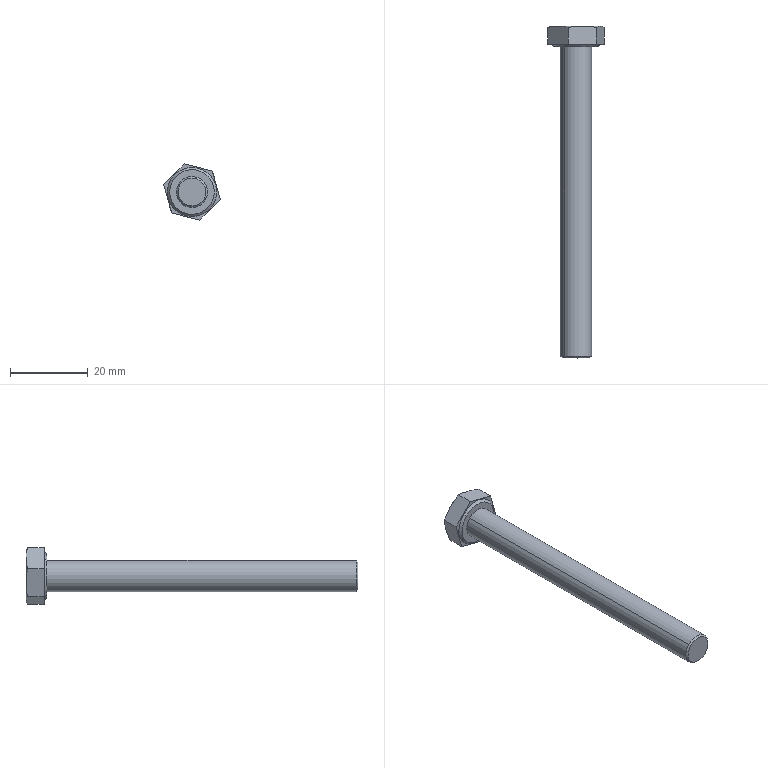Part | STEP file | 2026.6.15-Main Assembly图.sldasm-Part-28 | 1 solid | 22 faces | box 14.551 x 85.3 x 14.446 mm | volume 4774 mm3 | cone 10 | plane 10 | cylinder 2 | commonest cylinder face diameters 8 x2
STEP:
#1=CARTESIAN_POINT('',(-1049.783,460.541,3089.161));
#2=VERTEX_POINT('',#1);
#3=CARTESIAN_POINT('',(-1044.624,460.541,3084.139));
#4=VERTEX_POINT('',#3);
#5=CARTESIAN_POINT('',(-1047.204,460.541,3086.65));
#6=DIRECTION('',(0.,-1.,0.));
#7=DIRECTION('',(-0.7166,0.,0.6975));
#8=AXIS2_PLACEMENT_3D('',#5,#6,#7);
#9=CIRCLE('',#8,3.6);
#10=EDGE_CURVE('',#2,#4,#9,.T.);
#11=ORIENTED_EDGE('',*,*,#10,.F.);
#12=CARTESIAN_POINT('',(-1050.07,460.941,3089.44));
#13=VERTEX_POINT('',#12);
#14=CARTESIAN_POINT('',(-1049.783,460.541,3089.161));
#15=DIRECTION('',(-0.5067,0.7071,0.4932));
#16=VECTOR('',#15,1000.);
#17=LINE('',#14,#16);
#18=EDGE_CURVE('',#2,#13,#17,.T.);
#19=ORIENTED_EDGE('',*,*,#18,.T.);
#20=CARTESIAN_POINT('',(-1044.337,460.941,3083.86));
#21=VERTEX_POINT('',#20);
#22=CARTESIAN_POINT('',(-1047.204,460.941,3086.65));
#23=DIRECTION('',(0.,1.,0.));
#24=DIRECTION('',(-0.7166,0.,0.6975));
#25=AXIS2_PLACEMENT_3D('',#22,#23,#24);
#26=CIRCLE('',#25,4.);
#27=EDGE_CURVE('',#21,#13,#26,.T.);
#28=ORIENTED_EDGE('',*,*,#27,.F.);
#29=CARTESIAN_POINT('',(-1044.624,460.541,3084.139));
#30=DIRECTION('',(0.5067,0.7071,-0.4932));
#31=VECTOR('',#30,1000.);
#32=LINE('',#29,#31);
#33=EDGE_CURVE('',#4,#21,#32,.T.);
#34=ORIENTED_EDGE('',*,*,#33,.F.);
#35=EDGE_LOOP('',(#11,#19,#28,#34));
#36=FACE_OUTER_BOUND('',#35,.T.);
#37=CARTESIAN_POINT('',(-1047.204,460.541,3086.65));
#38=DIRECTION('',(0.,1.,0.));
#39=DIRECTION('',(-0.7166,0.,0.6975));
#40=AXIS2_PLACEMENT_3D('',#37,#38,#39);
#41=CONICAL_SURFACE('',#40,3.6,0.7854);
#42=ADVANCED_FACE('',(#36),#41,.T.);
#43=ORIENTED_EDGE('',*,*,#27,.T.);
#44=CARTESIAN_POINT('',(-1050.07,540.541,3089.44));
#45=VERTEX_POINT('',#44);
#46=CARTESIAN_POINT('',(-1050.07,460.541,3089.44));
#47=DIRECTION('',(0.,1.,0.));
#48=VECTOR('',#47,1000.);
#49=LINE('',#46,#48);
#50=EDGE_CURVE('',#13,#45,#49,.T.);
#51=ORIENTED_EDGE('',*,*,#50,.T.);
#52=CARTESIAN_POINT('',(-1044.337,540.541,3083.86));
#53=VERTEX_POINT('',#52);
#54=CARTESIAN_POINT('',(-1047.204,540.541,3086.65));
#55=DIRECTION('',(0.,-1.,0.));
#56=DIRECTION('',(0.7166,0.,-0.6975));
#57=AXIS2_PLACEMENT_3D('',#54,#55,#56);
#58=CIRCLE('',#57,4.);
#59=EDGE_CURVE('',#45,#53,#58,.T.);
#60=ORIENTED_EDGE('',*,*,#59,.T.);
#61=CARTESIAN_POINT('',(-1044.337,460.541,3083.86));
#62=DIRECTION('',(0.,1.,0.));
#63=VECTOR('',#62,1000.);
#64=LINE('',#61,#63);
#65=EDGE_CURVE('',#21,#53,#64,.T.);
#66=ORIENTED_EDGE('',*,*,#65,.F.);
#67=EDGE_LOOP('',(#43,#51,#60,#66));
#68=FACE_OUTER_BOUND('',#67,.T.);
#69=CARTESIAN_POINT('',(-1047.204,460.541,3086.65));
#70=DIRECTION('',(0.,1.,0.));
#71=DIRECTION('',(-0.7166,0.,0.6975));
#72=AXIS2_PLACEMENT_3D('',#69,#70,#71);
#73=CYLINDRICAL_SURFACE('',#72,4.);
#74=ADVANCED_FACE('',(#68),#73,.T.);
#75=CARTESIAN_POINT('',(-1043.094,540.541,3082.65));
#76=VERTEX_POINT('',#75);
#77=CARTESIAN_POINT('',(-1051.313,540.541,3090.65));
#78=VERTEX_POINT('',#77);
#79=CARTESIAN_POINT('',(-1047.204,540.541,3086.65));
#80=DIRECTION('',(0.,1.,0.));
#81=DIRECTION('',(0.7166,0.,-0.6975));
#82=AXIS2_PLACEMENT_3D('',#79,#80,#81);
#83=CIRCLE('',#82,5.735);
#84=EDGE_CURVE('',#76,#78,#83,.T.);
#85=ORIENTED_EDGE('',*,*,#84,.T.);
#86=CARTESIAN_POINT('',(-1051.743,541.141,3091.069));
#87=VERTEX_POINT('',#86);
#88=CARTESIAN_POINT('',(-1051.743,541.141,3091.069));
#89=DIRECTION('',(-0.5067,0.7071,0.4932));
#90=VECTOR('',#89,1000.);
#91=LINE('',#88,#90);
#92=EDGE_CURVE('',#78,#87,#91,.T.);
#93=ORIENTED_EDGE('',*,*,#92,.T.);
#94=CARTESIAN_POINT('',(-1042.664,541.141,3082.231));
#95=VERTEX_POINT('',#94);
#96=CARTESIAN_POINT('',(-1047.204,541.141,3086.65));
#97=DIRECTION('',(0.,1.,0.));
#98=DIRECTION('',(0.7166,0.,-0.6975));
#99=AXIS2_PLACEMENT_3D('',#96,#97,#98);
#100=CIRCLE('',#99,6.335);
#101=EDGE_CURVE('',#95,#87,#100,.T.);
#102=ORIENTED_EDGE('',*,*,#101,.F.);
#103=CARTESIAN_POINT('',(-1042.664,541.141,3082.231));
#104=DIRECTION('',(0.5067,0.7071,-0.4932));
#105=VECTOR('',#104,1000.);
#106=LINE('',#103,#105);
#107=EDGE_CURVE('',#76,#95,#106,.T.);
#108=ORIENTED_EDGE('',*,*,#107,.F.);
#109=EDGE_LOOP('',(#85,#93,#102,#108));
#110=FACE_OUTER_BOUND('',#109,.T.);
#111=CARTESIAN_POINT('',(-1047.204,541.141,3086.65));
#112=DIRECTION('',(0.,1.,0.));
#113=DIRECTION('',(-0.7166,0.,0.6975));
#114=AXIS2_PLACEMENT_3D('',#111,#112,#113);
#115=CONICAL_SURFACE('',#114,6.335,0.7854);
#116=ADVANCED_FACE('',(#110),#115,.T.);
#117=ORIENTED_EDGE('',*,*,#84,.F.);
#118=CARTESIAN_POINT('',(-1047.204,540.541,3086.65));
#119=DIRECTION('',(0.,1.,0.));
#120=DIRECTION('',(0.7166,0.,-0.6975));
#121=AXIS2_PLACEMENT_3D('',#118,#119,#120);
#122=CIRCLE('',#121,5.735);
#123=EDGE_CURVE('',#78,#76,#122,.T.);
#124=ORIENTED_EDGE('',*,*,#123,.F.);
#125=EDGE_LOOP('',(#117,#124));
#126=FACE_OUTER_BOUND('',#125,.T.);
#127=CARTESIAN_POINT('',(-1047.204,540.541,3086.65));
#128=DIRECTION('',(0.,-1.,0.));
#129=DIRECTION('',(0.7166,0.,-0.6975));
#130=AXIS2_PLACEMENT_3D('',#127,#128,#129);
#131=CIRCLE('',#130,4.);
#132=EDGE_CURVE('',#53,#45,#131,.T.);
#133=ORIENTED_EDGE('',*,*,#132,.F.);
#134=ORIENTED_EDGE('',*,*,#59,.F.);
#135=EDGE_LOOP('',(#133,#134));
#136=FACE_BOUND('',#135,.T.);
#137=CARTESIAN_POINT('',(-1037.888,540.541,3077.582));
#138=DIRECTION('',(0.,1.,0.));
#139=DIRECTION('',(-0.7166,0.,0.6975));
#140=AXIS2_PLACEMENT_3D('',#137,#138,#139);
#141=PLANE('',#140);
#142=ADVANCED_FACE('',(#126,#136),#141,.F.);
#143=CARTESIAN_POINT('',(-1041.968,545.475,3092.028));
#144=VERTEX_POINT('',#143);
#145=CARTESIAN_POINT('',(-1040.948,545.841,3088.417));
#146=VERTEX_POINT('',#145);
#147=CARTESIAN_POINT('',(-1041.968,545.475,3092.028));
#148=CARTESIAN_POINT('',(-1041.631,545.701,3090.834));
#149=CARTESIAN_POINT('',(-1041.292,545.841,3089.632));
#150=CARTESIAN_POINT('',(-1040.948,545.841,3088.417));
#151=B_SPLINE_CURVE_WITH_KNOTS('',3,(#147,#148,#149,#150),.UNSPECIFIED.,.F.,.F.,(4,4),(0.,0.003771),.UNSPECIFIED.);
#152=EDGE_CURVE('',#144,#146,#151,.T.);
#153=ORIENTED_EDGE('',*,*,#152,.F.);
#154=CARTESIAN_POINT('',(-1041.968,541.141,3092.028));
#155=VERTEX_POINT('',#154);
#156=CARTESIAN_POINT('',(-1041.968,540.541,3092.028));
#157=DIRECTION('',(0.,1.,0.));
#158=VECTOR('',#157,1000.);
#159=LINE('',#156,#158);
#160=EDGE_CURVE('',#155,#144,#159,.T.);
#161=ORIENTED_EDGE('',*,*,#160,.F.);
#162=CARTESIAN_POINT('',(-1039.928,541.141,3084.805));
#163=VERTEX_POINT('',#162);
#164=CARTESIAN_POINT('',(-1039.928,541.141,3084.805));
#165=DIRECTION('',(-0.2718,0.,0.9624));
#166=VECTOR('',#165,1000.);
#167=LINE('',#164,#166);
#168=EDGE_CURVE('',#163,#155,#167,.T.);
#169=ORIENTED_EDGE('',*,*,#168,.F.);
#170=CARTESIAN_POINT('',(-1039.928,545.475,3084.805));
#171=VERTEX_POINT('',#170);
#172=CARTESIAN_POINT('',(-1039.928,540.541,3084.805));
#173=DIRECTION('',(0.,1.,0.));
#174=VECTOR('',#173,1000.);
#175=LINE('',#172,#174);
#176=EDGE_CURVE('',#163,#171,#175,.T.);
#177=ORIENTED_EDGE('',*,*,#176,.T.);
#178=CARTESIAN_POINT('',(-1040.948,545.841,3088.417));
#179=CARTESIAN_POINT('',(-1040.605,545.841,3087.201));
#180=CARTESIAN_POINT('',(-1040.266,545.701,3085.999));
#181=CARTESIAN_POINT('',(-1039.928,545.475,3084.805));
#182=B_SPLINE_CURVE_WITH_KNOTS('',3,(#178,#179,#180,#181),.UNSPECIFIED.,.F.,.F.,(4,4),(0.,0.003771),.UNSPECIFIED.);
#183=EDGE_CURVE('',#146,#171,#182,.T.);
#184=ORIENTED_EDGE('',*,*,#183,.F.);
#185=EDGE_LOOP('',(#153,#161,#169,#177,#184));
#186=FACE_OUTER_BOUND('',#185,.T.);
#187=CARTESIAN_POINT('',(-1039.928,540.541,3084.805));
#188=DIRECTION('',(-0.9624,0.,-0.2718));
#189=DIRECTION('',(0.,-1.,0.));
#190=AXIS2_PLACEMENT_3D('',#187,#188,#189);
#191=PLANE('',#190);
#192=ADVANCED_FACE('',(#186),#191,.F.);
#193=CARTESIAN_POINT('',(-1049.244,545.475,3093.873));
#194=VERTEX_POINT('',#193);
#195=CARTESIAN_POINT('',(-1045.606,545.841,3092.951));
#196=VERTEX_POINT('',#195);
#197=CARTESIAN_POINT('',(-1049.244,545.475,3093.873));
#198=CARTESIAN_POINT('',(-1048.041,545.701,3093.568));
#199=CARTESIAN_POINT('',(-1046.83,545.841,3093.261));
#200=CARTESIAN_POINT('',(-1045.606,545.841,3092.951));
#201=B_SPLINE_CURVE_WITH_KNOTS('',3,(#197,#198,#199,#200),.UNSPECIFIED.,.F.,.F.,(4,4),(0.,0.003771),.UNSPECIFIED.);
#202=EDGE_CURVE('',#194,#196,#201,.T.);
#203=ORIENTED_EDGE('',*,*,#202,.F.);
#204=CARTESIAN_POINT('',(-1049.244,541.141,3093.873));
#205=VERTEX_POINT('',#204);
#206=CARTESIAN_POINT('',(-1049.244,540.541,3093.873));
#207=DIRECTION('',(0.,1.,0.));
#208=VECTOR('',#207,1000.);
#209=LINE('',#206,#208);
#210=EDGE_CURVE('',#205,#194,#209,.T.);
#211=ORIENTED_EDGE('',*,*,#210,.F.);
#212=CARTESIAN_POINT('',(-1041.968,541.141,3092.028));
#213=DIRECTION('',(-0.9693,0.,0.2458));
#214=VECTOR('',#213,1000.);
#215=LINE('',#212,#214);
#216=EDGE_CURVE('',#155,#205,#215,.T.);
#217=ORIENTED_EDGE('',*,*,#216,.F.);
#218=ORIENTED_EDGE('',*,*,#160,.T.);
#219=CARTESIAN_POINT('',(-1045.606,545.841,3092.951));
#220=CARTESIAN_POINT('',(-1044.382,545.841,3092.64));
#221=CARTESIAN_POINT('',(-1043.171,545.701,3092.333));
#222=CARTESIAN_POINT('',(-1041.968,545.475,3092.028));
#223=B_SPLINE_CURVE_WITH_KNOTS('',3,(#219,#220,#221,#222),.UNSPECIFIED.,.F.,.F.,(4,4),(0.,0.003771),.UNSPECIFIED.);
#224=EDGE_CURVE('',#196,#144,#223,.T.);
#225=ORIENTED_EDGE('',*,*,#224,.F.);
#226=EDGE_LOOP('',(#203,#211,#217,#218,#225));
#227=FACE_OUTER_BOUND('',#226,.T.);
#228=CARTESIAN_POINT('',(-1041.968,540.541,3092.028));
#229=DIRECTION('',(-0.2458,0.,-0.9693));
#230=DIRECTION('',(0.,1.,0.));
#231=AXIS2_PLACEMENT_3D('',#228,#229,#230);
#232=PLANE('',#231);
#233=ADVANCED_FACE('',(#227),#232,.F.);
#234=CARTESIAN_POINT('',(-1054.479,545.475,3088.495));
#235=VERTEX_POINT('',#234);
#236=CARTESIAN_POINT('',(-1051.861,545.841,3091.184));
#237=VERTEX_POINT('',#236);
#238=CARTESIAN_POINT('',(-1054.479,545.475,3088.495));
#239=CARTESIAN_POINT('',(-1053.614,545.701,3089.384));
#240=CARTESIAN_POINT('',(-1052.742,545.841,3090.279));
#241=CARTESIAN_POINT('',(-1051.861,545.841,3091.184));
#242=B_SPLINE_CURVE_WITH_KNOTS('',3,(#238,#239,#240,#241),.UNSPECIFIED.,.F.,.F.,(4,4),(0.,0.003771),.UNSPECIFIED.);
#243=EDGE_CURVE('',#235,#237,#242,.T.);
#244=ORIENTED_EDGE('',*,*,#243,.F.);
#245=CARTESIAN_POINT('',(-1054.479,541.141,3088.495));
#246=VERTEX_POINT('',#245);
#247=CARTESIAN_POINT('',(-1054.479,540.541,3088.495));
#248=DIRECTION('',(0.,1.,0.));
#249=VECTOR('',#248,1000.);
#250=LINE('',#247,#249);
#251=EDGE_CURVE('',#246,#235,#250,.T.);
#252=ORIENTED_EDGE('',*,*,#251,.F.);
#253=CARTESIAN_POINT('',(-1049.244,541.141,3093.873));
#254=DIRECTION('',(-0.6975,0.,-0.7166));
#255=VECTOR('',#254,1000.);
#256=LINE('',#253,#255);
#257=EDGE_CURVE('',#205,#246,#256,.T.);
#258=ORIENTED_EDGE('',*,*,#257,.F.);
#259=ORIENTED_EDGE('',*,*,#210,.T.);
#260=CARTESIAN_POINT('',(-1051.861,545.841,3091.184));
#261=CARTESIAN_POINT('',(-1050.98,545.841,3092.089));
#262=CARTESIAN_POINT('',(-1050.109,545.701,3092.984));
#263=CARTESIAN_POINT('',(-1049.244,545.475,3093.873));
#264=B_SPLINE_CURVE_WITH_KNOTS('',3,(#260,#261,#262,#263),.UNSPECIFIED.,.F.,.F.,(4,4),(0.,0.003771),.UNSPECIFIED.);
#265=EDGE_CURVE('',#237,#194,#264,.T.);
#266=ORIENTED_EDGE('',*,*,#265,.F.);
#267=EDGE_LOOP('',(#244,#252,#258,#259,#266));
#268=FACE_OUTER_BOUND('',#267,.T.);
#269=CARTESIAN_POINT('',(-1049.244,540.541,3093.873));
#270=DIRECTION('',(0.7166,0.,-0.6975));
#271=DIRECTION('',(-0.6975,0.,-0.7166));
#272=AXIS2_PLACEMENT_3D('',#269,#270,#271);
#273=PLANE('',#272);
#274=ADVANCED_FACE('',(#268),#273,.F.);
#275=CARTESIAN_POINT('',(-1052.439,545.475,3081.272));
#276=VERTEX_POINT('',#275);
#277=CARTESIAN_POINT('',(-1053.459,545.841,3084.883));
#278=VERTEX_POINT('',#277);
#279=CARTESIAN_POINT('',(-1052.439,545.475,3081.272));
#280=CARTESIAN_POINT('',(-1052.776,545.701,3082.466));
#281=CARTESIAN_POINT('',(-1053.116,545.841,3083.668));
#282=CARTESIAN_POINT('',(-1053.459,545.841,3084.883));
#283=B_SPLINE_CURVE_WITH_KNOTS('',3,(#279,#280,#281,#282),.UNSPECIFIED.,.F.,.F.,(4,4),(0.,0.003771),.UNSPECIFIED.);
#284=EDGE_CURVE('',#276,#278,#283,.T.);
#285=ORIENTED_EDGE('',*,*,#284,.F.);
#286=CARTESIAN_POINT('',(-1052.439,541.141,3081.272));
#287=VERTEX_POINT('',#286);
#288=CARTESIAN_POINT('',(-1052.439,540.541,3081.272));
#289=DIRECTION('',(0.,1.,0.));
#290=VECTOR('',#289,1000.);
#291=LINE('',#288,#290);
#292=EDGE_CURVE('',#287,#276,#291,.T.);
#293=ORIENTED_EDGE('',*,*,#292,.F.);
#294=CARTESIAN_POINT('',(-1054.479,541.141,3088.495));
#295=DIRECTION('',(0.2718,0.,-0.9624));
#296=VECTOR('',#295,1000.);
#297=LINE('',#294,#296);
#298=EDGE_CURVE('',#246,#287,#297,.T.);
#299=ORIENTED_EDGE('',*,*,#298,.F.);
#300=ORIENTED_EDGE('',*,*,#251,.T.);
#301=CARTESIAN_POINT('',(-1053.459,545.841,3084.883));
#302=CARTESIAN_POINT('',(-1053.802,545.841,3086.099));
#303=CARTESIAN_POINT('',(-1054.142,545.701,3087.301));
#304=CARTESIAN_POINT('',(-1054.479,545.475,3088.495));
#305=B_SPLINE_CURVE_WITH_KNOTS('',3,(#301,#302,#303,#304),.UNSPECIFIED.,.F.,.F.,(4,4),(0.,0.003771),.UNSPECIFIED.);
#306=EDGE_CURVE('',#278,#235,#305,.T.);
#307=ORIENTED_EDGE('',*,*,#306,.F.);
#308=EDGE_LOOP('',(#285,#293,#299,#300,#307));
#309=FACE_OUTER_BOUND('',#308,.T.);
#310=CARTESIAN_POINT('',(-1054.479,540.541,3088.495));
#311=DIRECTION('',(0.9624,0.,0.2718));
#312=DIRECTION('',(0.,-1.,0.));
#313=AXIS2_PLACEMENT_3D('',#310,#311,#312);
#314=PLANE('',#313);
#315=ADVANCED_FACE('',(#309),#314,.F.);
#316=CARTESIAN_POINT('',(-1045.164,545.475,3079.427));
#317=VERTEX_POINT('',#316);
#318=CARTESIAN_POINT('',(-1048.801,545.841,3080.349));
#319=VERTEX_POINT('',#318);
#320=CARTESIAN_POINT('',(-1045.164,545.475,3079.427));
#321=CARTESIAN_POINT('',(-1046.366,545.701,3079.732));
#322=CARTESIAN_POINT('',(-1047.577,545.841,3080.039));
#323=CARTESIAN_POINT('',(-1048.801,545.841,3080.349));
#324=B_SPLINE_CURVE_WITH_KNOTS('',3,(#320,#321,#322,#323),.UNSPECIFIED.,.F.,.F.,(4,4),(0.,0.003771),.UNSPECIFIED.);
#325=EDGE_CURVE('',#317,#319,#324,.T.);
#326=ORIENTED_EDGE('',*,*,#325,.F.);
#327=CARTESIAN_POINT('',(-1045.164,541.141,3079.427));
#328=VERTEX_POINT('',#327);
#329=CARTESIAN_POINT('',(-1045.164,540.541,3079.427));
#330=DIRECTION('',(0.,1.,0.));
#331=VECTOR('',#330,1000.);
#332=LINE('',#329,#331);
#333=EDGE_CURVE('',#328,#317,#332,.T.);
#334=ORIENTED_EDGE('',*,*,#333,.F.);
#335=CARTESIAN_POINT('',(-1052.439,541.141,3081.272));
#336=DIRECTION('',(0.9693,0.,-0.2458));
#337=VECTOR('',#336,1000.);
#338=LINE('',#335,#337);
#339=EDGE_CURVE('',#287,#328,#338,.T.);
#340=ORIENTED_EDGE('',*,*,#339,.F.);
#341=ORIENTED_EDGE('',*,*,#292,.T.);
#342=CARTESIAN_POINT('',(-1048.801,545.841,3080.349));
#343=CARTESIAN_POINT('',(-1050.025,545.841,3080.66));
#344=CARTESIAN_POINT('',(-1051.236,545.701,3080.967));
#345=CARTESIAN_POINT('',(-1052.439,545.475,3081.272));
#346=B_SPLINE_CURVE_WITH_KNOTS('',3,(#342,#343,#344,#345),.UNSPECIFIED.,.F.,.F.,(4,4),(0.,0.003771),.UNSPECIFIED.);
#347=EDGE_CURVE('',#319,#276,#346,.T.);
#348=ORIENTED_EDGE('',*,*,#347,.F.);
#349=EDGE_LOOP('',(#326,#334,#340,#341,#348));
#350=FACE_OUTER_BOUND('',#349,.T.);
#351=CARTESIAN_POINT('',(-1052.439,540.541,3081.272));
#352=DIRECTION('',(0.2458,0.,0.9693));
#353=DIRECTION('',(0.9693,0.,-0.2458));
#354=AXIS2_PLACEMENT_3D('',#351,#352,#353);
#355=PLANE('',#354);
#356=ADVANCED_FACE('',(#350),#355,.F.);
#357=CARTESIAN_POINT('',(-1042.546,545.841,3082.116));
#358=VERTEX_POINT('',#357);
#359=CARTESIAN_POINT('',(-1039.928,545.475,3084.805));
#360=CARTESIAN_POINT('',(-1040.794,545.701,3083.916));
#361=CARTESIAN_POINT('',(-1041.665,545.841,3083.021));
#362=CARTESIAN_POINT('',(-1042.546,545.841,3082.116));
#363=B_SPLINE_CURVE_WITH_KNOTS('',3,(#359,#360,#361,#362),.UNSPECIFIED.,.F.,.F.,(4,4),(0.,0.003771),.UNSPECIFIED.);
#364=EDGE_CURVE('',#171,#358,#363,.T.);
#365=ORIENTED_EDGE('',*,*,#364,.F.);
#366=ORIENTED_EDGE('',*,*,#176,.F.);
#367=CARTESIAN_POINT('',(-1045.164,541.141,3079.427));
#368=DIRECTION('',(0.6975,0.,0.7166));
#369=VECTOR('',#368,1000.);
#370=LINE('',#367,#369);
#371=EDGE_CURVE('',#328,#163,#370,.T.);
#372=ORIENTED_EDGE('',*,*,#371,.F.);
#373=ORIENTED_EDGE('',*,*,#333,.T.);
#374=CARTESIAN_POINT('',(-1042.546,545.841,3082.116));
#375=CARTESIAN_POINT('',(-1043.427,545.841,3081.211));
#376=CARTESIAN_POINT('',(-1044.298,545.701,3080.316));
#377=CARTESIAN_POINT('',(-1045.164,545.475,3079.427));
#378=B_SPLINE_CURVE_WITH_KNOTS('',3,(#374,#375,#376,#377),.UNSPECIFIED.,.F.,.F.,(4,4),(0.,0.003771),.UNSPECIFIED.);
#379=EDGE_CURVE('',#358,#317,#378,.T.);
#380=ORIENTED_EDGE('',*,*,#379,.F.);
#381=EDGE_LOOP('',(#365,#366,#372,#373,#380));
#382=FACE_OUTER_BOUND('',#381,.T.);
#383=CARTESIAN_POINT('',(-1045.164,540.541,3079.427));
#384=DIRECTION('',(-0.7166,0.,0.6975));
#385=DIRECTION('',(-0.6975,0.,-0.7166));
#386=AXIS2_PLACEMENT_3D('',#383,#384,#385);
#387=PLANE('',#386);
#388=ADVANCED_FACE('',(#382),#387,.F.);
#389=ORIENTED_EDGE('',*,*,#168,.T.);
#390=ORIENTED_EDGE('',*,*,#216,.T.);
#391=ORIENTED_EDGE('',*,*,#257,.T.);
#392=ORIENTED_EDGE('',*,*,#298,.T.);
#393=ORIENTED_EDGE('',*,*,#339,.T.);
#394=ORIENTED_EDGE('',*,*,#371,.T.);
#395=EDGE_LOOP('',(#389,#390,#391,#392,#393,#394));
#396=FACE_OUTER_BOUND('',#395,.T.);
#397=ORIENTED_EDGE('',*,*,#101,.T.);
#398=CARTESIAN_POINT('',(-1047.204,541.141,3086.65));
#399=DIRECTION('',(0.,1.,0.));
#400=DIRECTION('',(0.7166,0.,-0.6975));
#401=AXIS2_PLACEMENT_3D('',#398,#399,#400);
#402=CIRCLE('',#401,6.335);
#403=EDGE_CURVE('',#87,#95,#402,.T.);
#404=ORIENTED_EDGE('',*,*,#403,.T.);
#405=EDGE_LOOP('',(#397,#404));
#406=FACE_BOUND('',#405,.T.);
#407=CARTESIAN_POINT('',(-1051.623,541.141,3082.111));
#408=DIRECTION('',(0.,-1.,0.));
#409=DIRECTION('',(0.6975,0.,0.7166));
#410=AXIS2_PLACEMENT_3D('',#407,#408,#409);
#411=PLANE('',#410);
#412=ADVANCED_FACE('',(#396,#406),#411,.T.);
#413=ORIENTED_EDGE('',*,*,#92,.F.);
#414=ORIENTED_EDGE('',*,*,#123,.T.);
#415=ORIENTED_EDGE('',*,*,#107,.T.);
#416=ORIENTED_EDGE('',*,*,#403,.F.);
#417=EDGE_LOOP('',(#413,#414,#415,#416));
#418=FACE_OUTER_BOUND('',#417,.T.);
#419=CARTESIAN_POINT('',(-1047.204,541.141,3086.65));
#420=DIRECTION('',(0.,1.,0.));
#421=DIRECTION('',(-0.7166,0.,0.6975));
#422=AXIS2_PLACEMENT_3D('',#419,#420,#421);
#423=CONICAL_SURFACE('',#422,6.335,0.7854);
#424=ADVANCED_FACE('',(#418),#423,.T.);
#425=ORIENTED_EDGE('',*,*,#183,.T.);
#426=ORIENTED_EDGE('',*,*,#364,.T.);
#427=CARTESIAN_POINT('',(-1047.204,545.841,3086.65));
#428=DIRECTION('',(0.,1.,0.));
#429=DIRECTION('',(0.7166,0.,-0.6975));
#430=AXIS2_PLACEMENT_3D('',#427,#428,#429);
#431=CIRCLE('',#430,6.5);
#432=EDGE_CURVE('',#146,#358,#431,.T.);
#433=ORIENTED_EDGE('',*,*,#432,.F.);
#434=EDGE_LOOP('',(#425,#426,#433));
#435=FACE_OUTER_BOUND('',#434,.T.);
#436=CARTESIAN_POINT('',(-1047.204,545.841,3086.65));
#437=DIRECTION('',(0.,-1.,0.));
#438=DIRECTION('',(0.7166,0.,-0.6975));
#439=AXIS2_PLACEMENT_3D('',#436,#437,#438);
#440=CONICAL_SURFACE('',#439,6.5,1.222);
#441=ADVANCED_FACE('',(#435),#440,.T.);
#442=ORIENTED_EDGE('',*,*,#224,.T.);
#443=ORIENTED_EDGE('',*,*,#152,.T.);
#444=CARTESIAN_POINT('',(-1047.204,545.841,3086.65));
#445=DIRECTION('',(0.,1.,0.));
#446=DIRECTION('',(0.7166,0.,-0.6975));
#447=AXIS2_PLACEMENT_3D('',#444,#445,#446);
#448=CIRCLE('',#447,6.5);
#449=EDGE_CURVE('',#196,#146,#448,.T.);
#450=ORIENTED_EDGE('',*,*,#449,.F.);
#451=EDGE_LOOP('',(#442,#443,#450));
#452=FACE_OUTER_BOUND('',#451,.T.);
#453=CARTESIAN_POINT('',(-1047.204,545.841,3086.65));
#454=DIRECTION('',(0.,-1.,0.));
#455=DIRECTION('',(0.7166,0.,-0.6975));
#456=AXIS2_PLACEMENT_3D('',#453,#454,#455);
#457=CONICAL_SURFACE('',#456,6.5,1.222);
#458=ADVANCED_FACE('',(#452),#457,.T.);
#459=ORIENTED_EDGE('',*,*,#265,.T.);
#460=ORIENTED_EDGE('',*,*,#202,.T.);
#461=CARTESIAN_POINT('',(-1047.204,545.841,3086.65));
#462=DIRECTION('',(0.,1.,0.));
#463=DIRECTION('',(0.7166,0.,-0.6975));
#464=AXIS2_PLACEMENT_3D('',#461,#462,#463);
#465=CIRCLE('',#464,6.5);
#466=EDGE_CURVE('',#237,#196,#465,.T.);
#467=ORIENTED_EDGE('',*,*,#466,.F.);
#468=EDGE_LOOP('',(#459,#460,#467));
#469=FACE_OUTER_BOUND('',#468,.T.);
#470=CARTESIAN_POINT('',(-1047.204,545.841,3086.65));
#471=DIRECTION('',(0.,-1.,0.));
#472=DIRECTION('',(0.7166,0.,-0.6975));
#473=AXIS2_PLACEMENT_3D('',#470,#471,#472);
#474=CONICAL_SURFACE('',#473,6.5,1.222);
#475=ADVANCED_FACE('',(#469),#474,.T.);
#476=ORIENTED_EDGE('',*,*,#243,.T.);
#477=CARTESIAN_POINT('',(-1047.204,545.841,3086.65));
#478=DIRECTION('',(0.,1.,0.));
#479=DIRECTION('',(0.7166,0.,-0.6975));
#480=AXIS2_PLACEMENT_3D('',#477,#478,#479);
#481=CIRCLE('',#480,6.5);
#482=EDGE_CURVE('',#278,#237,#481,.T.);
#483=ORIENTED_EDGE('',*,*,#482,.F.);
#484=ORIENTED_EDGE('',*,*,#306,.T.);
#485=EDGE_LOOP('',(#476,#483,#484));
#486=FACE_OUTER_BOUND('',#485,.T.);
#487=CARTESIAN_POINT('',(-1047.204,545.841,3086.65));
#488=DIRECTION('',(0.,-1.,0.));
#489=DIRECTION('',(0.7166,0.,-0.6975));
#490=AXIS2_PLACEMENT_3D('',#487,#488,#489);
#491=CONICAL_SURFACE('',#490,6.5,1.222);
#492=ADVANCED_FACE('',(#486),#491,.T.);
#493=ORIENTED_EDGE('',*,*,#284,.T.);
#494=CARTESIAN_POINT('',(-1047.204,545.841,3086.65));
#495=DIRECTION('',(0.,1.,0.));
#496=DIRECTION('',(0.7166,0.,-0.6975));
#497=AXIS2_PLACEMENT_3D('',#494,#495,#496);
#498=CIRCLE('',#497,6.5);
#499=EDGE_CURVE('',#319,#278,#498,.T.);
#500=ORIENTED_EDGE('',*,*,#499,.F.);
#501=ORIENTED_EDGE('',*,*,#347,.T.);
#502=EDGE_LOOP('',(#493,#500,#501));
#503=FACE_OUTER_BOUND('',#502,.T.);
#504=CARTESIAN_POINT('',(-1047.204,545.841,3086.65));
#505=DIRECTION('',(0.,-1.,0.));
#506=DIRECTION('',(0.7166,0.,-0.6975));
#507=AXIS2_PLACEMENT_3D('',#504,#505,#506);
#508=CONICAL_SURFACE('',#507,6.5,1.222);
#509=ADVANCED_FACE('',(#503),#508,.T.);
#510=ORIENTED_EDGE('',*,*,#325,.T.);
#511=CARTESIAN_POINT('',(-1047.204,545.841,3086.65));
#512=DIRECTION('',(0.,1.,0.));
#513=DIRECTION('',(0.7166,0.,-0.6975));
#514=AXIS2_PLACEMENT_3D('',#511,#512,#513);
#515=CIRCLE('',#514,6.5);
#516=EDGE_CURVE('',#358,#319,#515,.T.);
#517=ORIENTED_EDGE('',*,*,#516,.F.);
#518=ORIENTED_EDGE('',*,*,#379,.T.);
#519=EDGE_LOOP('',(#510,#517,#518));
#520=FACE_OUTER_BOUND('',#519,.T.);
#521=CARTESIAN_POINT('',(-1047.204,545.841,3086.65));
#522=DIRECTION('',(0.,-1.,0.));
#523=DIRECTION('',(0.7166,0.,-0.6975));
#524=AXIS2_PLACEMENT_3D('',#521,#522,#523);
#525=CONICAL_SURFACE('',#524,6.5,1.222);
#526=ADVANCED_FACE('',(#520),#525,.T.);
#527=ORIENTED_EDGE('',*,*,#432,.T.);
#528=ORIENTED_EDGE('',*,*,#516,.T.);
#529=ORIENTED_EDGE('',*,*,#499,.T.);
#530=ORIENTED_EDGE('',*,*,#482,.T.);
#531=ORIENTED_EDGE('',*,*,#466,.T.);
#532=ORIENTED_EDGE('',*,*,#449,.T.);
#533=EDGE_LOOP('',(#527,#528,#529,#530,#531,#532));
#534=FACE_OUTER_BOUND('',#533,.T.);
#535=CARTESIAN_POINT('',(-1037.888,545.841,3077.582));
#536=DIRECTION('',(0.,1.,0.));
#537=DIRECTION('',(-0.7166,0.,0.6975));
#538=AXIS2_PLACEMENT_3D('',#535,#536,#537);
#539=PLANE('',#538);
#540=ADVANCED_FACE('',(#534),#539,.T.);
#541=ORIENTED_EDGE('',*,*,#50,.F.);
#542=CARTESIAN_POINT('',(-1047.204,460.941,3086.65));
#543=DIRECTION('',(0.,1.,0.));
#544=DIRECTION('',(-0.7166,0.,0.6975));
#545=AXIS2_PLACEMENT_3D('',#542,#543,#544);
#546=CIRCLE('',#545,4.);
#547=EDGE_CURVE('',#13,#21,#546,.T.);
#548=ORIENTED_EDGE('',*,*,#547,.T.);
#549=ORIENTED_EDGE('',*,*,#65,.T.);
#550=ORIENTED_EDGE('',*,*,#132,.T.);
#551=EDGE_LOOP('',(#541,#548,#549,#550));
#552=FACE_OUTER_BOUND('',#551,.T.);
#553=CARTESIAN_POINT('',(-1047.204,460.541,3086.65));
#554=DIRECTION('',(0.,1.,0.));
#555=DIRECTION('',(-0.7166,0.,0.6975));
#556=AXIS2_PLACEMENT_3D('',#553,#554,#555);
#557=CYLINDRICAL_SURFACE('',#556,4.);
#558=ADVANCED_FACE('',(#552),#557,.T.);
#559=CARTESIAN_POINT('',(-1047.204,460.541,3086.65));
#560=DIRECTION('',(0.,-1.,0.));
#561=DIRECTION('',(-0.7166,0.,0.6975));
#562=AXIS2_PLACEMENT_3D('',#559,#560,#561);
#563=CIRCLE('',#562,3.6);
#564=EDGE_CURVE('',#4,#2,#563,.T.);
#565=ORIENTED_EDGE('',*,*,#564,.T.);
#566=ORIENTED_EDGE('',*,*,#10,.T.);
#567=EDGE_LOOP('',(#565,#566));
#568=FACE_OUTER_BOUND('',#567,.T.);
#569=CARTESIAN_POINT('',(-1047.204,460.541,3086.65));
#570=DIRECTION('',(0.,-1.,0.));
#571=DIRECTION('',(0.6975,0.,0.7166));
#572=AXIS2_PLACEMENT_3D('',#569,#570,#571);
#573=PLANE('',#572);
#574=ADVANCED_FACE('',(#568),#573,.T.);
#575=ORIENTED_EDGE('',*,*,#18,.F.);
#576=ORIENTED_EDGE('',*,*,#564,.F.);
#577=ORIENTED_EDGE('',*,*,#33,.T.);
#578=ORIENTED_EDGE('',*,*,#547,.F.);
#579=EDGE_LOOP('',(#575,#576,#577,#578));
#580=FACE_OUTER_BOUND('',#579,.T.);
#581=CARTESIAN_POINT('',(-1047.204,460.541,3086.65));
#582=DIRECTION('',(0.,1.,0.));
#583=DIRECTION('',(-0.7166,0.,0.6975));
#584=AXIS2_PLACEMENT_3D('',#581,#582,#583);
#585=CONICAL_SURFACE('',#584,3.6,0.7854);
#586=ADVANCED_FACE('',(#580),#585,.T.);
#587=CLOSED_SHELL('',(#42,#74,#116,#142,#192,#233,#274,#315,#356,#388,#412,#424,#441,#458,#475,#492,#509,#526,#540,#558,#574,#586));
#588=MANIFOLD_SOLID_BREP('',#587);
#589=CARTESIAN_POINT('',(0.,0.,0.));
#590=DIRECTION('',(0.,0.,1.));
#591=DIRECTION('',(1.,0.,0.));
#592=AXIS2_PLACEMENT_3D('',#589,#590,#591);
#593=(LENGTH_UNIT()NAMED_UNIT(*)SI_UNIT(.MILLI.,.METRE.));
#594=UNCERTAINTY_MEASURE_WITH_UNIT(LENGTH_MEASURE(0.00001),#593,'','');
#595=(NAMED_UNIT(*)PLANE_ANGLE_UNIT()SI_UNIT($,.RADIAN.));
#596=(NAMED_UNIT(*)SI_UNIT($,.STERADIAN.)SOLID_ANGLE_UNIT());
#597=(GEOMETRIC_REPRESENTATION_CONTEXT(3)GLOBAL_UNCERTAINTY_ASSIGNED_CONTEXT((#594))GLOBAL_UNIT_ASSIGNED_CONTEXT((#593,#595,#596))REPRESENTATION_CONTEXT('',''));
#598=ADVANCED_BREP_SHAPE_REPRESENTATION('',(#588,#592),#597);